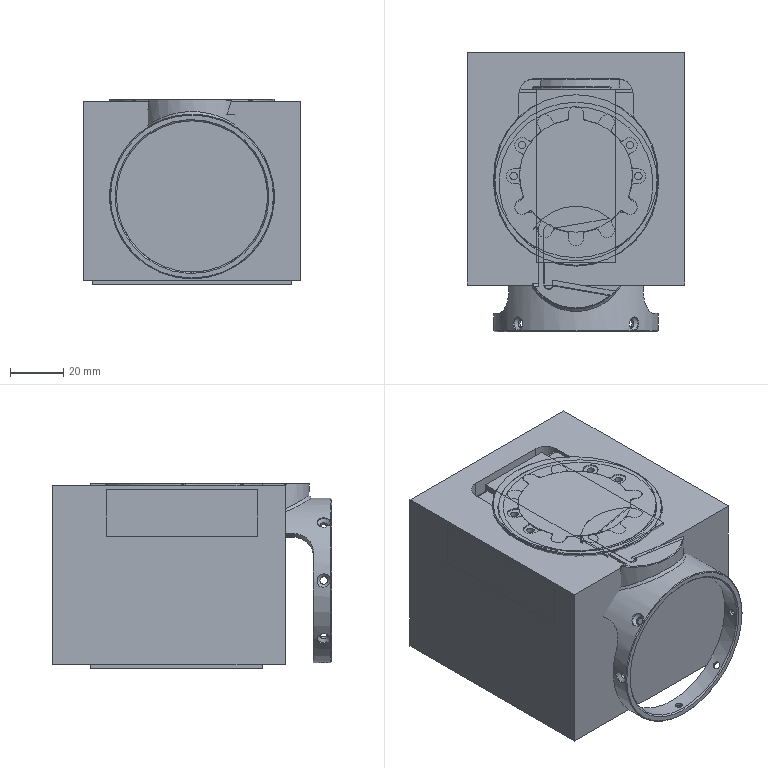NC program | NX | posted with a generic post | part box 82 x 105.2 x 70 mm
Whole program:
N10 G17 G21 G94 G90
(单向轮廓精光 , TOOL : 飞刀D50)
N12 T20 M6
N14 G53
N16 G17 G0 G90 X-40.2 Y-67.7 B0. C0. S4000 M3
N18 G43 Z10. H20
N20 Z2.133
N22 G94 G1 Z-0.867 F2000.
N24 G41 Y-32.5 D20
N26 Y32.5
N28 Y67.5
N30 G40
N32 Y67.7
N34 Z2.133
N36 G0 Z10.
N38 Y-67.7
N40 Z1.067
N42 G1 Z-1.933
N44 G41 Y-32.5
N46 Y32.5
N48 Y67.5
N50 G40
N52 Y67.7
N54 Z1.067
N56 G0 Z10.
N58 Y-67.7
N60 Z0.
N62 G1 Z-3.
N64 G41 Y-32.5
N66 Y32.5
N68 Y67.5
N70 G40
N72 Y67.7
N74 Z0.
N76 G0 Z10.
N78 X40.2
N80 Z2.133
N82 G1 Z-0.867
N84 G41 Y32.5
N86 Y-32.5
N88 Y-67.5
N90 G40
N92 Y-67.7
N94 Z2.133
N96 G0 Z10.
N98 Y67.7
N100 Z1.067
N102 G1 Z-1.933
N104 G41 Y32.5
N106 Y-32.5
N108 Y-67.5
N110 G40
N112 Y-67.7
N114 Z1.067
N116 G0 Z10.
N118 Y67.7
N120 Z0.
N122 G1 Z-3.
N124 G41 Y32.5
N126 Y-32.5
N128 Y-67.5
N130 G40
N132 Y-67.7
N134 Z0.
N136 G0 Z10.
(单向轮廓精光_COPY , TOOL : 飞刀D50)
N138 X-40.2
N140 Z0.
N142 G1 Z-3. F1000.
N144 G41 Y-32.5
N146 Y32.5
N148 Y67.5
N150 G40
N152 Y67.7
N154 Z0.
N156 G0 Z10.
N158 X40.2
N160 Z0.
N162 G1 Z-3.
N164 G41 Y32.5
N166 Y-32.5
N168 Y-67.5
N170 G40
N172 Y-67.7
N174 Z0.
N176 G0 Z10.
N178 M5
(单向轮廓精光_1 , TOOL : 光刀D10)
N180 T19 M6
N182 G53
N184 G17 G0 G90 X-20. Y-40.7 B0. C0. S8000 M3
N186 G43 Z10. H19
N188 Z0.
N190 G94 G1 Z-3. F1200.
N192 G41 Y-32.5 D19
N194 Y32.5
N196 Y40.5
N198 G40
N200 Y40.7
N202 Z0.
N204 G0 Z10.
N206 X20.
N208 Z0.
N210 G1 Z-3.
N212 G41 Y32.5
N214 Y-32.5
N216 Y-40.5
N218 G40
N220 Y-40.7
N222 Z0.
N224 G0 Z10.
N226 M5
(倒角刀D6._1 , TOOL : 倒角刀D6)
N228 T26 M6
N230 G53
N232 G17 G0 G90 X-16.2 Y-36.6 B0. C0. S7500 M3
N234 G43 Z10. H26
N236 Z1.5
N238 G94 G1 Z-1.5 F1200.
N240 G41 Y-32.5 D26
N242 Y32.5
N244 Y36.4
N246 G40
N248 Y36.6
N250 Z1.5
N252 G0 Z10.
N254 X16.2
N256 Z1.5
N258 G1 Z-1.5
N260 G41 Y32.5
N262 Y-32.5
N264 Y-36.4
N266 G40
N268 Y-36.6
N270 Z1.5
N272 G0 Z10.
N274 M5
N276 M2